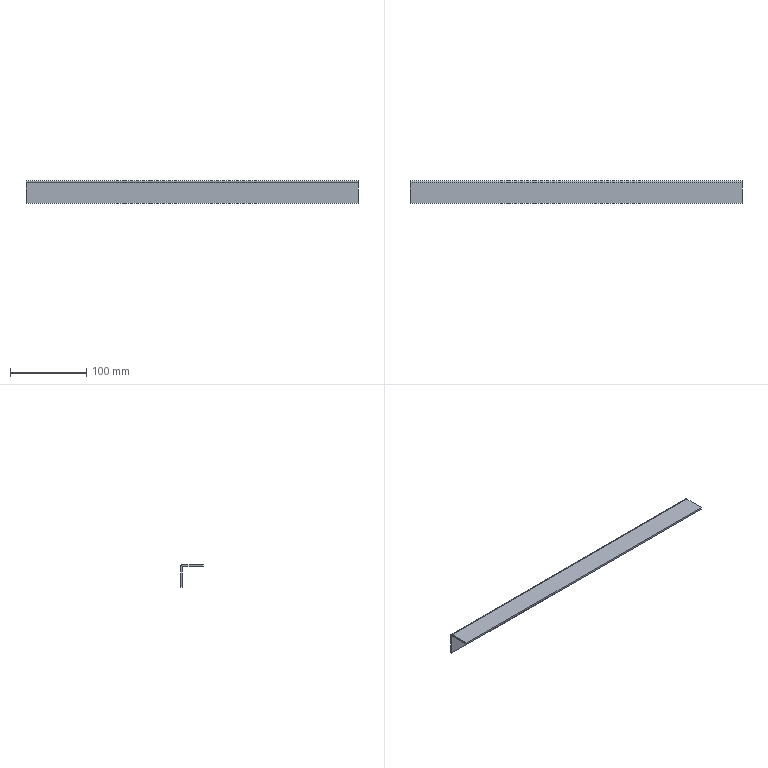Part | SolidWorks | features EdgeFlange 1, FlatPattern 1, SMBaseFlange 1, SheetMetal 1 | 1 solid | 14 faces | box 435.5 x 30 x 30 mm | volume 61785 mm3 | plane 12 | cylinder 2 | commonest cylinder face diameters 1 x1 6 x1
STEP:
#1=CARTESIAN_POINT('',(217.75,-15.,-2.5));
#2=VERTEX_POINT('',#1);
#3=CARTESIAN_POINT('',(217.75,12.,-2.5));
#4=VERTEX_POINT('',#3);
#5=CARTESIAN_POINT('',(217.75,15.,-2.5));
#6=DIRECTION('',(0.,1.,0.));
#7=VECTOR('',#6,1000.);
#8=LINE('',#5,#7);
#9=EDGE_CURVE('',#2,#4,#8,.T.);
#10=ORIENTED_EDGE('',*,*,#9,.T.);
#11=CARTESIAN_POINT('',(217.75,12.,0.));
#12=VERTEX_POINT('',#11);
#13=CARTESIAN_POINT('',(217.75,12.,-2.5));
#14=DIRECTION('',(0.,0.,1.));
#15=VECTOR('',#14,1000.);
#16=LINE('',#13,#15);
#17=EDGE_CURVE('',#4,#12,#16,.T.);
#18=ORIENTED_EDGE('',*,*,#17,.T.);
#19=CARTESIAN_POINT('',(217.75,-15.,0.));
#20=VERTEX_POINT('',#19);
#21=CARTESIAN_POINT('',(217.75,15.,0.));
#22=DIRECTION('',(0.,1.,0.));
#23=VECTOR('',#22,1000.);
#24=LINE('',#21,#23);
#25=EDGE_CURVE('',#20,#12,#24,.T.);
#26=ORIENTED_EDGE('',*,*,#25,.F.);
#27=CARTESIAN_POINT('',(217.75,-15.,-2.5));
#28=DIRECTION('',(0.,0.,1.));
#29=VECTOR('',#28,1000.);
#30=LINE('',#27,#29);
#31=EDGE_CURVE('',#2,#20,#30,.T.);
#32=ORIENTED_EDGE('',*,*,#31,.F.);
#33=EDGE_LOOP('',(#10,#18,#26,#32));
#34=FACE_OUTER_BOUND('',#33,.T.);
#35=CARTESIAN_POINT('',(217.75,15.,-2.5));
#36=DIRECTION('',(1.,0.,0.));
#37=DIRECTION('',(0.,0.,-1.));
#38=AXIS2_PLACEMENT_3D('',#35,#36,#37);
#39=PLANE('',#38);
#40=ADVANCED_FACE('',(#34),#39,.T.);
#41=CARTESIAN_POINT('',(-217.75,12.,-2.5));
#42=VERTEX_POINT('',#41);
#43=CARTESIAN_POINT('',(217.75,12.,-2.5));
#44=DIRECTION('',(-1.,0.,0.));
#45=VECTOR('',#44,1000.);
#46=LINE('',#43,#45);
#47=EDGE_CURVE('',#4,#42,#46,.T.);
#48=ORIENTED_EDGE('',*,*,#47,.F.);
#49=ORIENTED_EDGE('',*,*,#9,.F.);
#50=CARTESIAN_POINT('',(-217.75,-15.,-2.5));
#51=VERTEX_POINT('',#50);
#52=CARTESIAN_POINT('',(-217.75,-15.,-2.5));
#53=DIRECTION('',(1.,0.,0.));
#54=VECTOR('',#53,1000.);
#55=LINE('',#52,#54);
#56=EDGE_CURVE('',#51,#2,#55,.T.);
#57=ORIENTED_EDGE('',*,*,#56,.F.);
#58=CARTESIAN_POINT('',(-217.75,15.,-2.5));
#59=DIRECTION('',(0.,-1.,0.));
#60=VECTOR('',#59,1000.);
#61=LINE('',#58,#60);
#62=EDGE_CURVE('',#42,#51,#61,.T.);
#63=ORIENTED_EDGE('',*,*,#62,.F.);
#64=EDGE_LOOP('',(#48,#49,#57,#63));
#65=FACE_OUTER_BOUND('',#64,.T.);
#66=CARTESIAN_POINT('',(0.,0.,-2.5));
#67=DIRECTION('',(0.,0.,1.));
#68=DIRECTION('',(1.,0.,0.));
#69=AXIS2_PLACEMENT_3D('',#66,#67,#68);
#70=PLANE('',#69);
#71=ADVANCED_FACE('',(#65),#70,.F.);
#72=ORIENTED_EDGE('',*,*,#25,.T.);
#73=CARTESIAN_POINT('',(-217.75,12.,0.));
#74=VERTEX_POINT('',#73);
#75=CARTESIAN_POINT('',(217.75,12.,0.));
#76=DIRECTION('',(-1.,0.,0.));
#77=VECTOR('',#76,1000.);
#78=LINE('',#75,#77);
#79=EDGE_CURVE('',#12,#74,#78,.T.);
#80=ORIENTED_EDGE('',*,*,#79,.T.);
#81=CARTESIAN_POINT('',(-217.75,-15.,0.));
#82=VERTEX_POINT('',#81);
#83=CARTESIAN_POINT('',(-217.75,15.,0.));
#84=DIRECTION('',(0.,-1.,0.));
#85=VECTOR('',#84,1000.);
#86=LINE('',#83,#85);
#87=EDGE_CURVE('',#74,#82,#86,.T.);
#88=ORIENTED_EDGE('',*,*,#87,.T.);
#89=CARTESIAN_POINT('',(-217.75,-15.,0.));
#90=DIRECTION('',(1.,0.,0.));
#91=VECTOR('',#90,1000.);
#92=LINE('',#89,#91);
#93=EDGE_CURVE('',#82,#20,#92,.T.);
#94=ORIENTED_EDGE('',*,*,#93,.T.);
#95=EDGE_LOOP('',(#72,#80,#88,#94));
#96=FACE_OUTER_BOUND('',#95,.T.);
#97=CARTESIAN_POINT('',(0.,0.,0.));
#98=DIRECTION('',(0.,0.,1.));
#99=DIRECTION('',(1.,0.,0.));
#100=AXIS2_PLACEMENT_3D('',#97,#98,#99);
#101=PLANE('',#100);
#102=ADVANCED_FACE('',(#96),#101,.T.);
#103=ORIENTED_EDGE('',*,*,#93,.F.);
#104=CARTESIAN_POINT('',(-217.75,-15.,-2.5));
#105=DIRECTION('',(0.,0.,1.));
#106=VECTOR('',#105,1000.);
#107=LINE('',#104,#106);
#108=EDGE_CURVE('',#51,#82,#107,.T.);
#109=ORIENTED_EDGE('',*,*,#108,.F.);
#110=ORIENTED_EDGE('',*,*,#56,.T.);
#111=ORIENTED_EDGE('',*,*,#31,.T.);
#112=EDGE_LOOP('',(#103,#109,#110,#111));
#113=FACE_OUTER_BOUND('',#112,.T.);
#114=CARTESIAN_POINT('',(-217.75,-15.,-2.5));
#115=DIRECTION('',(0.,-1.,0.));
#116=DIRECTION('',(0.,0.,-1.));
#117=AXIS2_PLACEMENT_3D('',#114,#115,#116);
#118=PLANE('',#117);
#119=ADVANCED_FACE('',(#113),#118,.T.);
#120=CARTESIAN_POINT('',(-217.75,12.,-2.5));
#121=DIRECTION('',(0.,0.,1.));
#122=VECTOR('',#121,1000.);
#123=LINE('',#120,#122);
#124=EDGE_CURVE('',#42,#74,#123,.T.);
#125=ORIENTED_EDGE('',*,*,#124,.F.);
#126=ORIENTED_EDGE('',*,*,#62,.T.);
#127=ORIENTED_EDGE('',*,*,#108,.T.);
#128=ORIENTED_EDGE('',*,*,#87,.F.);
#129=EDGE_LOOP('',(#125,#126,#127,#128));
#130=FACE_OUTER_BOUND('',#129,.T.);
#131=CARTESIAN_POINT('',(-217.75,15.,-2.5));
#132=DIRECTION('',(-1.,0.,0.));
#133=DIRECTION('',(0.,0.,1.));
#134=AXIS2_PLACEMENT_3D('',#131,#132,#133);
#135=PLANE('',#134);
#136=ADVANCED_FACE('',(#130),#135,.T.);
#137=CARTESIAN_POINT('',(-217.75,12.5,-3.));
#138=VERTEX_POINT('',#137);
#139=CARTESIAN_POINT('',(-217.75,15.,-3.));
#140=VERTEX_POINT('',#139);
#141=CARTESIAN_POINT('',(-217.75,15.,-3.));
#142=DIRECTION('',(0.,1.,0.));
#143=VECTOR('',#142,1000.);
#144=LINE('',#141,#143);
#145=EDGE_CURVE('',#138,#140,#144,.T.);
#146=ORIENTED_EDGE('',*,*,#145,.F.);
#147=CARTESIAN_POINT('',(-217.75,12.,-3.));
#148=DIRECTION('',(-1.,0.,0.));
#149=DIRECTION('',(0.,0.,-1.));
#150=AXIS2_PLACEMENT_3D('',#147,#148,#149);
#151=CIRCLE('',#150,0.5);
#152=EDGE_CURVE('',#42,#138,#151,.T.);
#153=ORIENTED_EDGE('',*,*,#152,.F.);
#154=ORIENTED_EDGE('',*,*,#124,.T.);
#155=CARTESIAN_POINT('',(-217.75,12.,-3.));
#156=DIRECTION('',(-1.,0.,0.));
#157=DIRECTION('',(0.,0.,-1.));
#158=AXIS2_PLACEMENT_3D('',#155,#156,#157);
#159=CIRCLE('',#158,3.);
#160=EDGE_CURVE('',#74,#140,#159,.T.);
#161=ORIENTED_EDGE('',*,*,#160,.T.);
#162=EDGE_LOOP('',(#146,#153,#154,#161));
#163=FACE_OUTER_BOUND('',#162,.T.);
#164=CARTESIAN_POINT('',(-217.75,12.,-3.));
#165=DIRECTION('',(-1.,0.,0.));
#166=DIRECTION('',(0.,0.,1.));
#167=AXIS2_PLACEMENT_3D('',#164,#165,#166);
#168=PLANE('',#167);
#169=ADVANCED_FACE('',(#163),#168,.T.);
#170=CARTESIAN_POINT('',(217.75,12.5,-3.));
#171=VERTEX_POINT('',#170);
#172=CARTESIAN_POINT('',(217.75,12.,-3.));
#173=DIRECTION('',(1.,0.,0.));
#174=DIRECTION('',(0.,0.,-1.));
#175=AXIS2_PLACEMENT_3D('',#172,#173,#174);
#176=CIRCLE('',#175,0.5);
#177=EDGE_CURVE('',#171,#4,#176,.T.);
#178=ORIENTED_EDGE('',*,*,#177,.F.);
#179=CARTESIAN_POINT('',(217.75,15.,-3.));
#180=VERTEX_POINT('',#179);
#181=CARTESIAN_POINT('',(217.75,12.5,-3.));
#182=DIRECTION('',(0.,1.,0.));
#183=VECTOR('',#182,1000.);
#184=LINE('',#181,#183);
#185=EDGE_CURVE('',#171,#180,#184,.T.);
#186=ORIENTED_EDGE('',*,*,#185,.T.);
#187=CARTESIAN_POINT('',(217.75,12.,-3.));
#188=DIRECTION('',(1.,0.,0.));
#189=DIRECTION('',(0.,0.,-1.));
#190=AXIS2_PLACEMENT_3D('',#187,#188,#189);
#191=CIRCLE('',#190,3.);
#192=EDGE_CURVE('',#180,#12,#191,.T.);
#193=ORIENTED_EDGE('',*,*,#192,.T.);
#194=ORIENTED_EDGE('',*,*,#17,.F.);
#195=EDGE_LOOP('',(#178,#186,#193,#194));
#196=FACE_OUTER_BOUND('',#195,.T.);
#197=CARTESIAN_POINT('',(217.75,12.,-3.));
#198=DIRECTION('',(-1.,0.,0.));
#199=DIRECTION('',(0.,0.,1.));
#200=AXIS2_PLACEMENT_3D('',#197,#198,#199);
#201=PLANE('',#200);
#202=ADVANCED_FACE('',(#196),#201,.F.);
#203=ORIENTED_EDGE('',*,*,#79,.F.);
#204=ORIENTED_EDGE('',*,*,#192,.F.);
#205=CARTESIAN_POINT('',(0.,15.,-3.));
#206=DIRECTION('',(1.,0.,0.));
#207=VECTOR('',#206,1000.);
#208=LINE('',#205,#207);
#209=EDGE_CURVE('',#140,#180,#208,.T.);
#210=ORIENTED_EDGE('',*,*,#209,.F.);
#211=ORIENTED_EDGE('',*,*,#160,.F.);
#212=EDGE_LOOP('',(#203,#204,#210,#211));
#213=FACE_OUTER_BOUND('',#212,.T.);
#214=CARTESIAN_POINT('',(217.75,12.,-3.));
#215=DIRECTION('',(1.,0.,0.));
#216=DIRECTION('',(0.,1.,0.));
#217=AXIS2_PLACEMENT_3D('',#214,#215,#216);
#218=CYLINDRICAL_SURFACE('',#217,3.);
#219=ADVANCED_FACE('',(#213),#218,.T.);
#220=ORIENTED_EDGE('',*,*,#47,.T.);
#221=ORIENTED_EDGE('',*,*,#152,.T.);
#222=CARTESIAN_POINT('',(-217.75,12.5,-3.));
#223=DIRECTION('',(1.,0.,0.));
#224=VECTOR('',#223,1000.);
#225=LINE('',#222,#224);
#226=EDGE_CURVE('',#138,#171,#225,.T.);
#227=ORIENTED_EDGE('',*,*,#226,.T.);
#228=ORIENTED_EDGE('',*,*,#177,.T.);
#229=EDGE_LOOP('',(#220,#221,#227,#228));
#230=FACE_OUTER_BOUND('',#229,.T.);
#231=CARTESIAN_POINT('',(217.75,12.,-3.));
#232=DIRECTION('',(1.,0.,0.));
#233=DIRECTION('',(0.,1.,0.));
#234=AXIS2_PLACEMENT_3D('',#231,#232,#233);
#235=CYLINDRICAL_SURFACE('',#234,0.5);
#236=ADVANCED_FACE('',(#230),#235,.F.);
#237=CARTESIAN_POINT('',(217.75,15.,-30.));
#238=VERTEX_POINT('',#237);
#239=CARTESIAN_POINT('',(217.75,15.,-2.5));
#240=DIRECTION('',(0.,0.,1.));
#241=VECTOR('',#240,1000.);
#242=LINE('',#239,#241);
#243=EDGE_CURVE('',#238,#180,#242,.T.);
#244=ORIENTED_EDGE('',*,*,#243,.T.);
#245=ORIENTED_EDGE('',*,*,#185,.F.);
#246=CARTESIAN_POINT('',(217.75,12.5,-30.));
#247=VERTEX_POINT('',#246);
#248=CARTESIAN_POINT('',(217.75,12.5,0.));
#249=DIRECTION('',(0.,0.,1.));
#250=VECTOR('',#249,1000.);
#251=LINE('',#248,#250);
#252=EDGE_CURVE('',#247,#171,#251,.T.);
#253=ORIENTED_EDGE('',*,*,#252,.F.);
#254=CARTESIAN_POINT('',(217.75,15.,-30.));
#255=DIRECTION('',(0.,-1.,0.));
#256=VECTOR('',#255,1000.);
#257=LINE('',#254,#256);
#258=EDGE_CURVE('',#238,#247,#257,.T.);
#259=ORIENTED_EDGE('',*,*,#258,.F.);
#260=EDGE_LOOP('',(#244,#245,#253,#259));
#261=FACE_OUTER_BOUND('',#260,.T.);
#262=CARTESIAN_POINT('',(217.75,15.,-2.5));
#263=DIRECTION('',(1.,0.,0.));
#264=DIRECTION('',(0.,0.,-1.));
#265=AXIS2_PLACEMENT_3D('',#262,#263,#264);
#266=PLANE('',#265);
#267=ADVANCED_FACE('',(#261),#266,.T.);
#268=CARTESIAN_POINT('',(-217.75,12.5,-30.));
#269=VERTEX_POINT('',#268);
#270=CARTESIAN_POINT('',(-217.75,12.5,0.));
#271=DIRECTION('',(0.,0.,-1.));
#272=VECTOR('',#271,1000.);
#273=LINE('',#270,#272);
#274=EDGE_CURVE('',#138,#269,#273,.T.);
#275=ORIENTED_EDGE('',*,*,#274,.F.);
#276=ORIENTED_EDGE('',*,*,#145,.T.);
#277=CARTESIAN_POINT('',(-217.75,15.,-30.));
#278=VERTEX_POINT('',#277);
#279=CARTESIAN_POINT('',(-217.75,15.,-30.));
#280=DIRECTION('',(0.,0.,-1.));
#281=VECTOR('',#280,1000.);
#282=LINE('',#279,#281);
#283=EDGE_CURVE('',#140,#278,#282,.T.);
#284=ORIENTED_EDGE('',*,*,#283,.T.);
#285=CARTESIAN_POINT('',(-217.75,15.,-30.));
#286=DIRECTION('',(0.,-1.,0.));
#287=VECTOR('',#286,1000.);
#288=LINE('',#285,#287);
#289=EDGE_CURVE('',#278,#269,#288,.T.);
#290=ORIENTED_EDGE('',*,*,#289,.T.);
#291=EDGE_LOOP('',(#275,#276,#284,#290));
#292=FACE_OUTER_BOUND('',#291,.T.);
#293=CARTESIAN_POINT('',(-217.75,15.,-30.));
#294=DIRECTION('',(-1.,0.,0.));
#295=DIRECTION('',(0.,0.,1.));
#296=AXIS2_PLACEMENT_3D('',#293,#294,#295);
#297=PLANE('',#296);
#298=ADVANCED_FACE('',(#292),#297,.T.);
#299=ORIENTED_EDGE('',*,*,#283,.F.);
#300=ORIENTED_EDGE('',*,*,#209,.T.);
#301=ORIENTED_EDGE('',*,*,#243,.F.);
#302=CARTESIAN_POINT('',(217.75,15.,-30.));
#303=DIRECTION('',(1.,0.,0.));
#304=VECTOR('',#303,1000.);
#305=LINE('',#302,#304);
#306=EDGE_CURVE('',#278,#238,#305,.T.);
#307=ORIENTED_EDGE('',*,*,#306,.F.);
#308=EDGE_LOOP('',(#299,#300,#301,#307));
#309=FACE_OUTER_BOUND('',#308,.T.);
#310=CARTESIAN_POINT('',(0.,15.,0.));
#311=DIRECTION('',(0.,1.,0.));
#312=DIRECTION('',(0.,0.,1.));
#313=AXIS2_PLACEMENT_3D('',#310,#311,#312);
#314=PLANE('',#313);
#315=ADVANCED_FACE('',(#309),#314,.T.);
#316=ORIENTED_EDGE('',*,*,#226,.F.);
#317=ORIENTED_EDGE('',*,*,#274,.T.);
#318=CARTESIAN_POINT('',(0.,12.5,-30.));
#319=DIRECTION('',(1.,0.,0.));
#320=VECTOR('',#319,1000.);
#321=LINE('',#318,#320);
#322=EDGE_CURVE('',#269,#247,#321,.T.);
#323=ORIENTED_EDGE('',*,*,#322,.T.);
#324=ORIENTED_EDGE('',*,*,#252,.T.);
#325=EDGE_LOOP('',(#316,#317,#323,#324));
#326=FACE_OUTER_BOUND('',#325,.T.);
#327=CARTESIAN_POINT('',(0.,12.5,0.));
#328=DIRECTION('',(0.,1.,0.));
#329=DIRECTION('',(0.,0.,1.));
#330=AXIS2_PLACEMENT_3D('',#327,#328,#329);
#331=PLANE('',#330);
#332=ADVANCED_FACE('',(#326),#331,.F.);
#333=ORIENTED_EDGE('',*,*,#322,.F.);
#334=ORIENTED_EDGE('',*,*,#289,.F.);
#335=ORIENTED_EDGE('',*,*,#306,.T.);
#336=ORIENTED_EDGE('',*,*,#258,.T.);
#337=EDGE_LOOP('',(#333,#334,#335,#336));
#338=FACE_OUTER_BOUND('',#337,.T.);
#339=CARTESIAN_POINT('',(217.75,15.,-30.));
#340=DIRECTION('',(0.,0.,-1.));
#341=DIRECTION('',(0.,1.,0.));
#342=AXIS2_PLACEMENT_3D('',#339,#340,#341);
#343=PLANE('',#342);
#344=ADVANCED_FACE('',(#338),#343,.T.);
#345=CLOSED_SHELL('',(#40,#71,#102,#119,#136,#169,#202,#219,#236,#267,#298,#315,#332,#344));
#346=MANIFOLD_SOLID_BREP('',#345);
#347=CARTESIAN_POINT('',(0.,0.,0.));
#348=DIRECTION('',(0.,0.,1.));
#349=DIRECTION('',(1.,0.,0.));
#350=AXIS2_PLACEMENT_3D('',#347,#348,#349);
#351=(LENGTH_UNIT()NAMED_UNIT(*)SI_UNIT(.MILLI.,.METRE.));
#352=UNCERTAINTY_MEASURE_WITH_UNIT(LENGTH_MEASURE(0.00001),#351,'','');
#353=(NAMED_UNIT(*)PLANE_ANGLE_UNIT()SI_UNIT($,.RADIAN.));
#354=(NAMED_UNIT(*)SI_UNIT($,.STERADIAN.)SOLID_ANGLE_UNIT());
#355=(GEOMETRIC_REPRESENTATION_CONTEXT(3)GLOBAL_UNCERTAINTY_ASSIGNED_CONTEXT((#352))GLOBAL_UNIT_ASSIGNED_CONTEXT((#351,#353,#354))REPRESENTATION_CONTEXT('',''));
#356=ADVANCED_BREP_SHAPE_REPRESENTATION('',(#346,#350),#355);